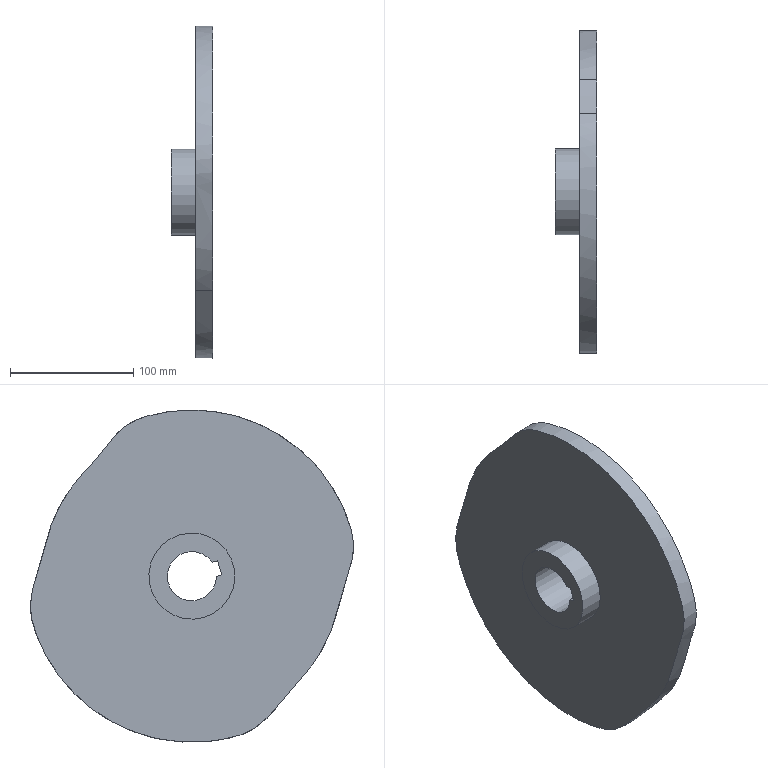Part | NX | features 146X000 2 | 1 solid | 11 faces | box 34 x 262.59 x 269.999 mm | volume 781015 mm3 | plane 6 | spline 3 | cylinder 2 | commonest cylinder face diameters 40 x1 70 x1
STEP:
#1=CARTESIAN_POINT('',(-21.5,-143.231,-819.079));
#2=VERTEX_POINT('',#1);
#3=CARTESIAN_POINT('',(-21.5,-138.999,-820.357));
#4=VERTEX_POINT('',#3);
#5=CARTESIAN_POINT('',(-21.5,-143.231,-819.079));
#6=DIRECTION('',(0.,0.9573,-0.2891));
#7=VECTOR('',#6,1000.);
#8=LINE('',#5,#7);
#9=EDGE_CURVE('',#2,#4,#8,.T.);
#10=ORIENTED_EDGE('',*,*,#9,.F.);
#11=CARTESIAN_POINT('',(12.5,-143.231,-819.079));
#12=VERTEX_POINT('',#11);
#13=CARTESIAN_POINT('',(-21.5,-143.231,-819.079));
#14=DIRECTION('',(1.,0.,0.));
#15=VECTOR('',#14,1000.);
#16=LINE('',#13,#15);
#17=EDGE_CURVE('',#2,#12,#16,.T.);
#18=ORIENTED_EDGE('',*,*,#17,.T.);
#19=CARTESIAN_POINT('',(12.5,-138.999,-820.357));
#20=VERTEX_POINT('',#19);
#21=CARTESIAN_POINT('',(12.5,-143.231,-819.079));
#22=DIRECTION('',(0.,0.9573,-0.2891));
#23=VECTOR('',#22,1000.);
#24=LINE('',#21,#23);
#25=EDGE_CURVE('',#12,#20,#24,.T.);
#26=ORIENTED_EDGE('',*,*,#25,.T.);
#27=CARTESIAN_POINT('',(-21.5,-138.999,-820.357));
#28=DIRECTION('',(1.,0.,0.));
#29=VECTOR('',#28,1000.);
#30=LINE('',#27,#29);
#31=EDGE_CURVE('',#4,#20,#30,.T.);
#32=ORIENTED_EDGE('',*,*,#31,.F.);
#33=EDGE_LOOP('',(#10,#18,#26,#32));
#34=FACE_BOUND('',#33,.T.);
#35=CARTESIAN_POINT('',(12.5,-143.231,-819.079));
#36=DIRECTION('',(0.,-0.2891,-0.9573));
#37=DIRECTION('',(0.,-0.9573,0.2891));
#38=AXIS2_PLACEMENT_3D('',#35,#36,#37);
#39=PLANE('',#38);
#40=ADVANCED_FACE('',(#34),#39,.F.);
#41=CARTESIAN_POINT('',(-21.5,-139.762,-807.591));
#42=VERTEX_POINT('',#41);
#43=CARTESIAN_POINT('',(-21.5,-139.762,-807.591));
#44=DIRECTION('',(0.,-0.2891,-0.9573));
#45=VECTOR('',#44,1000.);
#46=LINE('',#43,#45);
#47=EDGE_CURVE('',#42,#2,#46,.T.);
#48=ORIENTED_EDGE('',*,*,#47,.F.);
#49=CARTESIAN_POINT('',(12.5,-139.762,-807.591));
#50=VERTEX_POINT('',#49);
#51=CARTESIAN_POINT('',(-21.5,-139.762,-807.591));
#52=DIRECTION('',(1.,0.,0.));
#53=VECTOR('',#52,1000.);
#54=LINE('',#51,#53);
#55=EDGE_CURVE('',#42,#50,#54,.T.);
#56=ORIENTED_EDGE('',*,*,#55,.T.);
#57=CARTESIAN_POINT('',(12.5,-139.762,-807.591));
#58=DIRECTION('',(0.,-0.2891,-0.9573));
#59=VECTOR('',#58,1000.);
#60=LINE('',#57,#59);
#61=EDGE_CURVE('',#50,#12,#60,.T.);
#62=ORIENTED_EDGE('',*,*,#61,.T.);
#63=ORIENTED_EDGE('',*,*,#17,.F.);
#64=EDGE_LOOP('',(#48,#56,#62,#63));
#65=FACE_BOUND('',#64,.T.);
#66=CARTESIAN_POINT('',(12.5,-139.762,-807.591));
#67=DIRECTION('',(0.,-0.9573,0.2891));
#68=DIRECTION('',(-1.,0.,0.));
#69=AXIS2_PLACEMENT_3D('',#66,#67,#68);
#70=PLANE('',#69);
#71=ADVANCED_FACE('',(#65),#70,.F.);
#72=CARTESIAN_POINT('',(12.5,-135.529,-808.87));
#73=VERTEX_POINT('',#72);
#74=CARTESIAN_POINT('',(12.5,-135.529,-808.87));
#75=DIRECTION('',(0.,-0.9573,0.2891));
#76=VECTOR('',#75,1000.);
#77=LINE('',#74,#76);
#78=EDGE_CURVE('',#73,#50,#77,.T.);
#79=ORIENTED_EDGE('',*,*,#78,.T.);
#80=ORIENTED_EDGE('',*,*,#55,.F.);
#81=CARTESIAN_POINT('',(-21.5,-135.529,-808.87));
#82=VERTEX_POINT('',#81);
#83=CARTESIAN_POINT('',(-21.5,-135.529,-808.87));
#84=DIRECTION('',(0.,-0.9573,0.2891));
#85=VECTOR('',#84,1000.);
#86=LINE('',#83,#85);
#87=EDGE_CURVE('',#82,#42,#86,.T.);
#88=ORIENTED_EDGE('',*,*,#87,.F.);
#89=CARTESIAN_POINT('',(12.5,-135.529,-808.87));
#90=DIRECTION('',(-1.,0.,0.));
#91=VECTOR('',#90,1000.);
#92=LINE('',#89,#91);
#93=EDGE_CURVE('',#73,#82,#92,.T.);
#94=ORIENTED_EDGE('',*,*,#93,.F.);
#95=EDGE_LOOP('',(#79,#80,#88,#94));
#96=FACE_BOUND('',#95,.T.);
#97=CARTESIAN_POINT('',(12.5,-139.762,-807.591));
#98=DIRECTION('',(0.,0.2891,0.9573));
#99=DIRECTION('',(0.,0.9573,-0.2891));
#100=AXIS2_PLACEMENT_3D('',#97,#98,#99);
#101=PLANE('',#100);
#102=ADVANCED_FACE('',(#96),#101,.F.);
#103=CARTESIAN_POINT('',(-1.5,-129.119,-853.635));
#104=VERTEX_POINT('',#103);
#105=CARTESIAN_POINT('',(-1.5,-119.,-820.129));
#106=DIRECTION('',(1.,0.,0.));
#107=DIRECTION('',(0.,-0.2891,-0.9573));
#108=AXIS2_PLACEMENT_3D('',#105,#106,#107);
#109=CIRCLE('',#108,35.);
#110=EDGE_CURVE('',#104,#104,#109,.T.);
#111=ORIENTED_EDGE('',*,*,#110,.F.);
#112=EDGE_LOOP('',(#111));
#113=FACE_BOUND('',#112,.T.);
#114=CARTESIAN_POINT('',(-21.5,-108.881,-786.624));
#115=VERTEX_POINT('',#114);
#116=CARTESIAN_POINT('',(-21.5,-119.,-820.129));
#117=DIRECTION('',(-1.,0.,0.));
#118=DIRECTION('',(0.,0.2891,0.9573));
#119=AXIS2_PLACEMENT_3D('',#116,#117,#118);
#120=CIRCLE('',#119,35.);
#121=EDGE_CURVE('',#115,#115,#120,.T.);
#122=ORIENTED_EDGE('',*,*,#121,.F.);
#123=EDGE_LOOP('',(#122));
#124=FACE_BOUND('',#123,.T.);
#125=CARTESIAN_POINT('',(-21.5,-119.,-820.129));
#126=DIRECTION('',(1.,0.,0.));
#127=DIRECTION('',(0.,0.2891,0.9573));
#128=AXIS2_PLACEMENT_3D('',#125,#126,#127);
#129=CYLINDRICAL_SURFACE('',#128,35.);
#130=ADVANCED_FACE('',(#113,#124),#129,.T.);
#131=ORIENTED_EDGE('',*,*,#47,.T.);
#132=ORIENTED_EDGE('',*,*,#9,.T.);
#133=CARTESIAN_POINT('',(-21.5,-119.,-820.129));
#134=DIRECTION('',(1.,0.,0.));
#135=DIRECTION('',(0.,-0.9999,-0.01138));
#136=AXIS2_PLACEMENT_3D('',#133,#134,#135);
#137=CIRCLE('',#136,20.);
#138=EDGE_CURVE('',#4,#82,#137,.T.);
#139=ORIENTED_EDGE('',*,*,#138,.T.);
#140=ORIENTED_EDGE('',*,*,#87,.T.);
#141=EDGE_LOOP('',(#131,#132,#139,#140));
#142=FACE_BOUND('',#141,.T.);
#143=ORIENTED_EDGE('',*,*,#121,.T.);
#144=EDGE_LOOP('',(#143));
#145=FACE_BOUND('',#144,.T.);
#146=CARTESIAN_POINT('',(-21.5,-119.,-820.129));
#147=DIRECTION('',(-1.,0.,0.));
#148=DIRECTION('',(0.,-0.2891,-0.9573));
#149=AXIS2_PLACEMENT_3D('',#146,#147,#148);
#150=PLANE('',#149);
#151=ADVANCED_FACE('',(#142,#145),#150,.T.);
#152=ORIENTED_EDGE('',*,*,#138,.F.);
#153=ORIENTED_EDGE('',*,*,#31,.T.);
#154=CARTESIAN_POINT('',(12.5,-119.,-820.129));
#155=DIRECTION('',(-1.,0.,0.));
#156=DIRECTION('',(0.,-0.2891,-0.9573));
#157=AXIS2_PLACEMENT_3D('',#154,#155,#156);
#158=CIRCLE('',#157,20.);
#159=EDGE_CURVE('',#73,#20,#158,.T.);
#160=ORIENTED_EDGE('',*,*,#159,.F.);
#161=ORIENTED_EDGE('',*,*,#93,.T.);
#162=EDGE_LOOP('',(#152,#153,#160,#161));
#163=FACE_BOUND('',#162,.T.);
#164=CARTESIAN_POINT('',(-1.5,-119.,-820.129));
#165=DIRECTION('',(1.,0.,0.));
#166=DIRECTION('',(0.,0.2891,0.9573));
#167=AXIS2_PLACEMENT_3D('',#164,#165,#166);
#168=CYLINDRICAL_SURFACE('',#167,20.);
#169=ADVANCED_FACE('',(#163),#168,.F.);
#170=ORIENTED_EDGE('',*,*,#25,.F.);
#171=ORIENTED_EDGE('',*,*,#61,.F.);
#172=ORIENTED_EDGE('',*,*,#78,.F.);
#173=ORIENTED_EDGE('',*,*,#159,.T.);
#174=EDGE_LOOP('',(#170,#171,#172,#173));
#175=FACE_BOUND('',#174,.T.);
#176=CARTESIAN_POINT('',(12.5,-55.289,-707.283));
#177=VERTEX_POINT('',#176);
#178=CARTESIAN_POINT('',(12.5,-210.557,-900.047));
#179=VERTEX_POINT('',#178);
#180=CARTESIAN_POINT('',(12.5,-210.557,-900.047));
#181=CARTESIAN_POINT('',(12.5,-215.628,-894.239));
#182=CARTESIAN_POINT('',(12.5,-222.402,-884.799));
#183=CARTESIAN_POINT('',(12.5,-229.525,-871.101));
#184=CARTESIAN_POINT('',(12.5,-233.877,-860.369));
#185=CARTESIAN_POINT('',(12.5,-236.603,-851.114));
#186=CARTESIAN_POINT('',(12.5,-238.326,-843.598));
#187=CARTESIAN_POINT('',(12.5,-240.291,-836.142));
#188=CARTESIAN_POINT('',(12.5,-242.992,-826.89));
#189=CARTESIAN_POINT('',(12.5,-245.919,-817.711));
#190=CARTESIAN_POINT('',(12.5,-248.427,-810.413));
#191=CARTESIAN_POINT('',(12.5,-249.773,-804.781));
#192=CARTESIAN_POINT('',(12.5,-250.436,-799.023));
#193=CARTESIAN_POINT('',(12.5,-250.459,-793.232));
#194=CARTESIAN_POINT('',(12.5,-249.844,-787.468));
#195=CARTESIAN_POINT('',(12.5,-248.527,-781.829));
#196=CARTESIAN_POINT('',(12.5,-246.734,-776.328));
#197=CARTESIAN_POINT('',(12.5,-244.086,-769.086));
#198=CARTESIAN_POINT('',(12.5,-240.183,-760.263));
#199=CARTESIAN_POINT('',(12.5,-232.763,-746.73));
#200=CARTESIAN_POINT('',(12.5,-221.361,-731.099));
#201=CARTESIAN_POINT('',(12.5,-204.681,-714.949));
#202=CARTESIAN_POINT('',(12.5,-185.491,-701.879));
#203=CARTESIAN_POINT('',(12.5,-164.354,-692.273));
#204=CARTESIAN_POINT('',(12.5,-141.888,-686.412));
#205=CARTESIAN_POINT('',(12.5,-122.608,-684.792));
#206=CARTESIAN_POINT('',(12.5,-107.189,-685.481));
#207=CARTESIAN_POINT('',(12.5,-95.708,-686.986));
#208=CARTESIAN_POINT('',(12.5,-84.41,-689.462));
#209=CARTESIAN_POINT('',(12.5,-73.316,-692.896));
#210=CARTESIAN_POINT('',(12.5,-63.345,-698.946));
#211=CARTESIAN_POINT('',(12.5,-57.75,-704.315));
#212=CARTESIAN_POINT('',(12.5,-55.289,-707.283));
#213=B_SPLINE_CURVE_WITH_KNOTS('',3,(#180,#181,#182,#183,#184,#185,#186,#187,#188,#189,#190,#191,#192,#193,#194,#195,#196,#197,#198,#199,#200,#201,#202,#203,#204,#205,#206,#207,#208,#209,#210,#211,#212),.UNSPECIFIED.,.F.,.F.,(4,1,1,1,1,1,1,1,1,1,1,1,1,1,1,1,1,1,1,1,1,1,1,1,1,1,1,1,1,1,4),(0.,0.0625,0.09375,0.125,0.1562,0.1719,0.1875,0.2188,0.25,0.2656,0.2812,0.2969,0.3125,0.3281,0.3438,0.3594,0.375,0.4062,0.4375,0.5,0.5625,0.625,0.6875,0.75,0.8125,0.8438,0.875,0.9062,0.9375,0.9688,1.),.UNSPECIFIED.);
#214=EDGE_CURVE('',#177,#179,#213,.F.);
#215=ORIENTED_EDGE('',*,*,#214,.T.);
#216=CARTESIAN_POINT('',(12.5,-28.192,-739.361));
#217=VERTEX_POINT('',#216);
#218=CARTESIAN_POINT('',(12.5,-28.192,-739.361));
#219=CARTESIAN_POINT('',(12.5,-22.457,-745.808));
#220=CARTESIAN_POINT('',(12.5,-14.889,-756.399));
#221=CARTESIAN_POINT('',(12.5,-7.211,-771.882));
#222=CARTESIAN_POINT('',(12.5,-3.46,-782.011));
#223=CARTESIAN_POINT('',(12.5,-1.129,-790.322));
#224=CARTESIAN_POINT('',(12.5,0.8153,-798.73));
#225=CARTESIAN_POINT('',(12.5,3.97,-809.049));
#226=CARTESIAN_POINT('',(12.5,8.02,-821.337));
#227=CARTESIAN_POINT('',(12.5,11.36,-833.86));
#228=CARTESIAN_POINT('',(12.5,12.469,-844.644));
#229=CARTESIAN_POINT('',(12.5,11.752,-853.272));
#230=CARTESIAN_POINT('',(12.5,10.214,-859.571));
#231=CARTESIAN_POINT('',(12.5,8.118,-865.696));
#232=CARTESIAN_POINT('',(12.5,5.031,-873.754));
#233=CARTESIAN_POINT('',(12.5,0.4236,-883.52));
#234=CARTESIAN_POINT('',(12.5,-6.192,-894.661));
#235=CARTESIAN_POINT('',(12.5,-16.394,-908.605));
#236=CARTESIAN_POINT('',(12.5,-31.568,-924.078));
#237=CARTESIAN_POINT('',(12.5,-52.981,-938.835));
#238=CARTESIAN_POINT('',(12.5,-76.814,-949.242));
#239=CARTESIAN_POINT('',(12.5,-97.963,-953.968));
#240=CARTESIAN_POINT('',(12.5,-115.19,-955.283));
#241=CARTESIAN_POINT('',(12.5,-128.143,-955.022));
#242=CARTESIAN_POINT('',(12.5,-141.019,-953.545));
#243=CARTESIAN_POINT('',(12.5,-151.558,-951.228));
#244=CARTESIAN_POINT('',(12.5,-159.879,-948.915));
#245=CARTESIAN_POINT('',(12.5,-167.825,-945.483));
#246=CARTESIAN_POINT('',(12.5,-176.675,-939.179));
#247=CARTESIAN_POINT('',(12.5,-185.649,-929.812));
#248=CARTESIAN_POINT('',(12.5,-193.715,-919.69));
#249=CARTESIAN_POINT('',(12.5,-201.826,-909.605));
#250=CARTESIAN_POINT('',(12.5,-207.604,-903.192));
#251=CARTESIAN_POINT('',(12.5,-210.557,-900.047));
#252=B_SPLINE_CURVE_WITH_KNOTS('',3,(#218,#219,#220,#221,#222,#223,#224,#225,#226,#227,#228,#229,#230,#231,#232,#233,#234,#235,#236,#237,#238,#239,#240,#241,#242,#243,#244,#245,#246,#247,#248,#249,#250,#251),.UNSPECIFIED.,.F.,.F.,(4,1,1,1,1,1,1,1,1,1,1,1,1,1,1,1,1,1,1,1,1,1,1,1,1,1,1,1,1,1,1,4),(0.,0.0625,0.09375,0.125,0.1406,0.1562,0.1875,0.2188,0.25,0.2812,0.2969,0.3125,0.3281,0.3438,0.375,0.4062,0.4375,0.5,0.5625,0.625,0.6875,0.7188,0.75,0.7812,0.8125,0.8281,0.8438,0.875,0.9062,0.9375,0.9688,1.),.UNSPECIFIED.);
#253=EDGE_CURVE('',#179,#217,#252,.F.);
#254=ORIENTED_EDGE('',*,*,#253,.T.);
#255=CARTESIAN_POINT('',(12.5,-55.289,-707.283));
#256=CARTESIAN_POINT('',(12.5,-46.692,-718.331));
#257=CARTESIAN_POINT('',(12.5,-37.848,-729.212));
#258=CARTESIAN_POINT('',(12.5,-28.192,-739.361));
#259=B_SPLINE_CURVE_WITH_KNOTS('',3,(#255,#256,#257,#258),.UNSPECIFIED.,.F.,.F.,(4,4),(0.,1.),.UNSPECIFIED.);
#260=EDGE_CURVE('',#217,#177,#259,.F.);
#261=ORIENTED_EDGE('',*,*,#260,.T.);
#262=EDGE_LOOP('',(#215,#254,#261));
#263=FACE_BOUND('',#262,.T.);
#264=CARTESIAN_POINT('',(12.5,-258.55,-814.638));
#265=DIRECTION('',(-1.,0.,0.));
#266=DIRECTION('',(0.,-0.2891,-0.9573));
#267=AXIS2_PLACEMENT_3D('',#264,#265,#266);
#268=PLANE('',#267);
#269=ADVANCED_FACE('',(#175,#263),#268,.F.);
#270=ORIENTED_EDGE('',*,*,#253,.F.);
#271=CARTESIAN_POINT('',(-1.5,-210.557,-900.047));
#272=VERTEX_POINT('',#271);
#273=CARTESIAN_POINT('',(12.96,-210.557,-900.047));
#274=DIRECTION('',(-1.,0.,0.));
#275=VECTOR('',#274,1000.);
#276=LINE('',#273,#275);
#277=EDGE_CURVE('',#272,#179,#276,.F.);
#278=ORIENTED_EDGE('',*,*,#277,.F.);
#279=CARTESIAN_POINT('',(-1.5,-28.192,-739.361));
#280=VERTEX_POINT('',#279);
#281=CARTESIAN_POINT('',(-1.5,-210.557,-900.047));
#282=CARTESIAN_POINT('',(-1.5,-207.605,-903.192));
#283=CARTESIAN_POINT('',(-1.5,-201.825,-909.604));
#284=CARTESIAN_POINT('',(-1.5,-193.716,-919.69));
#285=CARTESIAN_POINT('',(-1.5,-185.649,-929.812));
#286=CARTESIAN_POINT('',(-1.5,-176.676,-939.179));
#287=CARTESIAN_POINT('',(-1.5,-167.825,-945.482));
#288=CARTESIAN_POINT('',(-1.5,-159.88,-948.917));
#289=CARTESIAN_POINT('',(-1.5,-151.557,-951.228));
#290=CARTESIAN_POINT('',(-1.5,-141.019,-953.545));
#291=CARTESIAN_POINT('',(-1.5,-128.143,-955.022));
#292=CARTESIAN_POINT('',(-1.5,-115.189,-955.283));
#293=CARTESIAN_POINT('',(-1.5,-97.961,-953.968));
#294=CARTESIAN_POINT('',(-1.5,-76.812,-949.241));
#295=CARTESIAN_POINT('',(-1.5,-52.98,-938.835));
#296=CARTESIAN_POINT('',(-1.5,-31.567,-924.077));
#297=CARTESIAN_POINT('',(-1.5,-16.394,-908.604));
#298=CARTESIAN_POINT('',(-1.5,-6.192,-894.66));
#299=CARTESIAN_POINT('',(-1.5,0.4238,-883.52));
#300=CARTESIAN_POINT('',(-1.5,5.032,-873.754));
#301=CARTESIAN_POINT('',(-1.5,8.118,-865.696));
#302=CARTESIAN_POINT('',(-1.5,10.217,-859.571));
#303=CARTESIAN_POINT('',(-1.5,11.752,-853.272));
#304=CARTESIAN_POINT('',(-1.5,12.469,-844.644));
#305=CARTESIAN_POINT('',(-1.5,11.36,-833.859));
#306=CARTESIAN_POINT('',(-1.5,8.02,-821.336));
#307=CARTESIAN_POINT('',(-1.5,3.97,-809.049));
#308=CARTESIAN_POINT('',(-1.5,0.8134,-798.73));
#309=CARTESIAN_POINT('',(-1.5,-1.13,-790.322));
#310=CARTESIAN_POINT('',(-1.5,-3.46,-782.011));
#311=CARTESIAN_POINT('',(-1.5,-7.211,-771.882));
#312=CARTESIAN_POINT('',(-1.5,-14.889,-756.399));
#313=CARTESIAN_POINT('',(-1.5,-22.457,-745.808));
#314=CARTESIAN_POINT('',(-1.5,-28.192,-739.361));
#315=B_SPLINE_CURVE_WITH_KNOTS('',3,(#281,#282,#283,#284,#285,#286,#287,#288,#289,#290,#291,#292,#293,#294,#295,#296,#297,#298,#299,#300,#301,#302,#303,#304,#305,#306,#307,#308,#309,#310,#311,#312,#313,#314),.UNSPECIFIED.,.F.,.F.,(4,1,1,1,1,1,1,1,1,1,1,1,1,1,1,1,1,1,1,1,1,1,1,1,1,1,1,1,1,1,1,4),(0.,0.03125,0.0625,0.09375,0.125,0.1562,0.1719,0.1875,0.2188,0.25,0.2812,0.3125,0.375,0.4375,0.5,0.5625,0.5938,0.625,0.6562,0.6719,0.6875,0.7031,0.7188,0.75,0.7812,0.8125,0.8438,0.8594,0.875,0.9062,0.9375,1.),.UNSPECIFIED.);
#316=EDGE_CURVE('',#280,#272,#315,.F.);
#317=ORIENTED_EDGE('',*,*,#316,.F.);
#318=CARTESIAN_POINT('',(12.96,-28.192,-739.361));
#319=DIRECTION('',(-1.,0.,0.));
#320=VECTOR('',#319,1000.);
#321=LINE('',#318,#320);
#322=EDGE_CURVE('',#280,#217,#321,.F.);
#323=ORIENTED_EDGE('',*,*,#322,.T.);
#324=EDGE_LOOP('',(#270,#278,#317,#323));
#325=FACE_BOUND('',#324,.T.);
#326=CARTESIAN_POINT('',(12.5,-28.192,-739.361));
#327=CARTESIAN_POINT('',(-1.5,-28.192,-739.361));
#328=CARTESIAN_POINT('',(12.5,-22.772,-745.455));
#329=CARTESIAN_POINT('',(-1.5,-22.772,-745.455));
#330=CARTESIAN_POINT('',(12.5,-15.496,-755.509));
#331=CARTESIAN_POINT('',(-1.5,-15.496,-755.509));
#332=CARTESIAN_POINT('',(12.5,-7.956,-770.227));
#333=CARTESIAN_POINT('',(-1.5,-7.956,-770.227));
#334=CARTESIAN_POINT('',(12.5,-4.229,-779.831));
#335=CARTESIAN_POINT('',(-1.5,-4.229,-779.831));
#336=CARTESIAN_POINT('',(12.5,-1.82,-787.656));
#337=CARTESIAN_POINT('',(-1.5,-1.82,-787.656));
#338=CARTESIAN_POINT('',(12.5,-0.405,-793.602));
#339=CARTESIAN_POINT('',(-1.5,-0.405,-793.602));
#340=CARTESIAN_POINT('',(12.5,1.116,-799.529));
#341=CARTESIAN_POINT('',(-1.5,1.116,-799.529));
#342=CARTESIAN_POINT('',(12.5,3.433,-807.345));
#343=CARTESIAN_POINT('',(-1.5,3.433,-807.345));
#344=CARTESIAN_POINT('',(12.5,6.621,-817.038));
#345=CARTESIAN_POINT('',(-1.5,6.621,-817.038));
#346=CARTESIAN_POINT('',(12.5,10.143,-828.727));
#347=CARTESIAN_POINT('',(-1.5,10.143,-828.727));
#348=CARTESIAN_POINT('',(12.5,11.998,-838.828));
#349=CARTESIAN_POINT('',(-1.5,11.998,-838.828));
#350=CARTESIAN_POINT('',(12.5,12.271,-846.909));
#351=CARTESIAN_POINT('',(-1.5,12.271,-846.909));
#352=CARTESIAN_POINT('',(12.5,11.771,-853.026));
#353=CARTESIAN_POINT('',(-1.5,11.771,-853.026));
#354=CARTESIAN_POINT('',(12.5,10.378,-859.029));
#355=CARTESIAN_POINT('',(-1.5,10.378,-859.029));
#356=CARTESIAN_POINT('',(12.5,7.74,-866.863));
#357=CARTESIAN_POINT('',(-1.5,7.74,-866.863));
#358=CARTESIAN_POINT('',(12.5,3.793,-876.75));
#359=CARTESIAN_POINT('',(-1.5,3.793,-876.75));
#360=CARTESIAN_POINT('',(12.5,-2.309,-888.442));
#361=CARTESIAN_POINT('',(-1.5,-2.309,-888.442));
#362=CARTESIAN_POINT('',(12.5,-12.196,-903.583));
#363=CARTESIAN_POINT('',(-1.5,-12.196,-903.583));
#364=CARTESIAN_POINT('',(12.5,-27.872,-921.093));
#365=CARTESIAN_POINT('',(-1.5,-27.872,-921.093));
#366=CARTESIAN_POINT('',(12.5,-51.286,-938.117));
#367=CARTESIAN_POINT('',(-1.5,-51.286,-938.117));
#368=CARTESIAN_POINT('',(12.5,-77.88,-949.785));
#369=CARTESIAN_POINT('',(-1.5,-77.88,-949.785));
#370=CARTESIAN_POINT('',(12.5,-101.127,-954.5));
#371=CARTESIAN_POINT('',(-1.5,-101.127,-954.5));
#372=CARTESIAN_POINT('',(12.5,-119.427,-955.354));
#373=CARTESIAN_POINT('',(-1.5,-119.427,-955.354));
#374=CARTESIAN_POINT('',(12.5,-132.808,-954.636));
#375=CARTESIAN_POINT('',(-1.5,-132.808,-954.636));
#376=CARTESIAN_POINT('',(12.5,-143.516,-953.009));
#377=CARTESIAN_POINT('',(-1.5,-143.516,-953.009));
#378=CARTESIAN_POINT('',(12.5,-151.748,-951.136));
#379=CARTESIAN_POINT('',(-1.5,-151.748,-951.136));
#380=CARTESIAN_POINT('',(12.5,-157.76,-949.537));
#381=CARTESIAN_POINT('',(-1.5,-157.76,-949.537));
#382=CARTESIAN_POINT('',(12.5,-163.513,-947.468));
#383=CARTESIAN_POINT('',(-1.5,-163.513,-947.468));
#384=CARTESIAN_POINT('',(12.5,-170.642,-943.635));
#385=CARTESIAN_POINT('',(-1.5,-170.642,-943.635));
#386=CARTESIAN_POINT('',(12.5,-178.706,-937.247));
#387=CARTESIAN_POINT('',(-1.5,-178.706,-937.247));
#388=CARTESIAN_POINT('',(12.5,-186.94,-928.233));
#389=CARTESIAN_POINT('',(-1.5,-186.94,-928.233));
#390=CARTESIAN_POINT('',(12.5,-194.567,-918.616));
#391=CARTESIAN_POINT('',(-1.5,-194.567,-918.616));
#392=CARTESIAN_POINT('',(12.5,-200.969,-910.663));
#393=CARTESIAN_POINT('',(-1.5,-200.969,-910.663));
#394=CARTESIAN_POINT('',(12.5,-206.404,-904.557));
#395=CARTESIAN_POINT('',(-1.5,-206.404,-904.557));
#396=CARTESIAN_POINT('',(12.5,-209.213,-901.587));
#397=CARTESIAN_POINT('',(-1.5,-209.213,-901.587));
#398=CARTESIAN_POINT('',(12.5,-210.557,-900.047));
#399=CARTESIAN_POINT('',(-1.5,-210.557,-900.047));
#400=B_SPLINE_SURFACE_WITH_KNOTS('',3,1,((#326,#327),(#328,#329),(#330,#331),(#332,#333),(#334,#335),(#336,#337),(#338,#339),(#340,#341),(#342,#343),(#344,#345),(#346,#347),(#348,#349),(#350,#351),(#352,#353),(#354,#355),(#356,#357),(#358,#359),(#360,#361),(#362,#363),(#364,#365),(#366,#367),(#368,#369),(#370,#371),(#372,#373),(#374,#375),(#376,#377),(#378,#379),(#380,#381),(#382,#383),(#384,#385),(#386,#387),(#388,#389),(#390,#391),(#392,#393),(#394,#395),(#396,#397),(#398,#399)),.SURF_OF_LINEAR_EXTRUSION.,.F.,.F.,.F.,(4,1,1,1,1,1,1,1,1,1,1,1,1,1,1,1,1,1,1,1,1,1,1,1,1,1,1,1,1,1,1,1,1,1,4),(2,2),(0.01026,0.0709,0.1012,0.1315,0.1467,0.1619,0.177,0.1922,0.2225,0.2528,0.2832,0.2983,0.3135,0.3286,0.3438,0.3741,0.4045,0.4348,0.4954,0.5561,0.6167,0.6774,0.7077,0.738,0.7683,0.7835,0.7987,0.8138,0.829,0.8593,0.8896,0.9199,0.9503,0.9654,0.9806),(0.,1.),.UNSPECIFIED.);
#401=ADVANCED_FACE('',(#325),#400,.T.);
#402=ORIENTED_EDGE('',*,*,#260,.F.);
#403=ORIENTED_EDGE('',*,*,#322,.F.);
#404=CARTESIAN_POINT('',(-1.5,-55.289,-707.283));
#405=VERTEX_POINT('',#404);
#406=CARTESIAN_POINT('',(-1.5,-28.192,-739.361));
#407=CARTESIAN_POINT('',(-1.5,-37.848,-729.212));
#408=CARTESIAN_POINT('',(-1.5,-46.692,-718.331));
#409=CARTESIAN_POINT('',(-1.5,-55.289,-707.283));
#410=B_SPLINE_CURVE_WITH_KNOTS('',3,(#406,#407,#408,#409),.UNSPECIFIED.,.F.,.F.,(4,4),(0.,1.),.UNSPECIFIED.);
#411=EDGE_CURVE('',#405,#280,#410,.F.);
#412=ORIENTED_EDGE('',*,*,#411,.F.);
#413=CARTESIAN_POINT('',(12.96,-55.289,-707.283));
#414=DIRECTION('',(-1.,0.,0.));
#415=VECTOR('',#414,1000.);
#416=LINE('',#413,#415);
#417=EDGE_CURVE('',#177,#405,#416,.T.);
#418=ORIENTED_EDGE('',*,*,#417,.F.);
#419=EDGE_LOOP('',(#402,#403,#412,#418));
#420=FACE_BOUND('',#419,.T.);
#421=CARTESIAN_POINT('',(12.5,-55.289,-707.283));
#422=CARTESIAN_POINT('',(-1.5,-55.289,-707.283));
#423=CARTESIAN_POINT('',(12.5,-54.177,-708.63));
#424=CARTESIAN_POINT('',(-1.5,-54.177,-708.63));
#425=CARTESIAN_POINT('',(12.5,-52.051,-711.419));
#426=CARTESIAN_POINT('',(-1.5,-52.051,-711.419));
#427=CARTESIAN_POINT('',(12.5,-47.694,-716.899));
#428=CARTESIAN_POINT('',(-1.5,-47.694,-716.899));
#429=CARTESIAN_POINT('',(12.5,-42.178,-723.693));
#430=CARTESIAN_POINT('',(-1.5,-42.178,-723.693));
#431=CARTESIAN_POINT('',(12.5,-35.355,-731.674));
#432=CARTESIAN_POINT('',(-1.5,-35.355,-731.674));
#433=CARTESIAN_POINT('',(12.5,-30.52,-736.745));
#434=CARTESIAN_POINT('',(-1.5,-30.52,-736.745));
#435=CARTESIAN_POINT('',(12.5,-28.192,-739.361));
#436=CARTESIAN_POINT('',(-1.5,-28.192,-739.361));
#437=B_SPLINE_SURFACE_WITH_KNOTS('',3,1,((#421,#422),(#423,#424),(#425,#426),(#427,#428),(#429,#430),(#431,#432),(#433,#434),(#435,#436)),.SURF_OF_LINEAR_EXTRUSION.,.F.,.F.,.F.,(4,1,1,1,1,4),(2,2),(0.009829,0.1324,0.2549,0.5,0.7451,0.9902),(0.,1.),.UNSPECIFIED.);
#438=ADVANCED_FACE('',(#420),#437,.T.);
#439=CARTESIAN_POINT('',(-1.5,-55.289,-707.283));
#440=CARTESIAN_POINT('',(-1.5,-57.75,-704.315));
#441=CARTESIAN_POINT('',(-1.5,-63.345,-698.947));
#442=CARTESIAN_POINT('',(-1.5,-73.314,-692.896));
#443=CARTESIAN_POINT('',(-1.5,-84.409,-689.474));
#444=CARTESIAN_POINT('',(-1.5,-95.704,-686.985));
#445=CARTESIAN_POINT('',(-1.5,-107.185,-685.482));
#446=CARTESIAN_POINT('',(-1.5,-122.604,-684.794));
#447=CARTESIAN_POINT('',(-1.5,-141.885,-686.413));
#448=CARTESIAN_POINT('',(-1.5,-164.351,-692.273));
#449=CARTESIAN_POINT('',(-1.5,-185.489,-701.878));
#450=CARTESIAN_POINT('',(-1.5,-204.68,-714.947));
#451=CARTESIAN_POINT('',(-1.5,-221.359,-731.098));
#452=CARTESIAN_POINT('',(-1.5,-232.762,-746.73));
#453=CARTESIAN_POINT('',(-1.5,-240.182,-760.264));
#454=CARTESIAN_POINT('',(-1.5,-244.093,-769.085));
#455=CARTESIAN_POINT('',(-1.5,-246.724,-776.332));
#456=CARTESIAN_POINT('',(-1.5,-248.544,-781.825));
#457=CARTESIAN_POINT('',(-1.5,-249.837,-787.471));
#458=CARTESIAN_POINT('',(-1.5,-250.461,-793.231));
#459=CARTESIAN_POINT('',(-1.5,-250.437,-799.023));
#460=CARTESIAN_POINT('',(-1.5,-249.771,-804.779));
#461=CARTESIAN_POINT('',(-1.5,-248.431,-810.415));
#462=CARTESIAN_POINT('',(-1.5,-245.915,-817.707));
#463=CARTESIAN_POINT('',(-1.5,-242.998,-826.89));
#464=CARTESIAN_POINT('',(-1.5,-240.278,-836.138));
#465=CARTESIAN_POINT('',(-1.5,-238.337,-843.6));
#466=CARTESIAN_POINT('',(-1.5,-236.602,-851.112));
#467=CARTESIAN_POINT('',(-1.5,-233.876,-860.368));
#468=CARTESIAN_POINT('',(-1.5,-229.523,-871.1));
#469=CARTESIAN_POINT('',(-1.5,-222.403,-884.798));
#470=CARTESIAN_POINT('',(-1.5,-215.627,-894.238));
#471=CARTESIAN_POINT('',(-1.5,-210.557,-900.047));
#472=B_SPLINE_CURVE_WITH_KNOTS('',3,(#439,#440,#441,#442,#443,#444,#445,#446,#447,#448,#449,#450,#451,#452,#453,#454,#455,#456,#457,#458,#459,#460,#461,#462,#463,#464,#465,#466,#467,#468,#469,#470,#471),.UNSPECIFIED.,.F.,.F.,(4,1,1,1,1,1,1,1,1,1,1,1,1,1,1,1,1,1,1,1,1,1,1,1,1,1,1,1,1,1,4),(0.,0.03125,0.0625,0.09375,0.125,0.1562,0.1875,0.25,0.3125,0.375,0.4375,0.5,0.5625,0.5938,0.625,0.6406,0.6562,0.6719,0.6875,0.7031,0.7188,0.7344,0.75,0.7812,0.8125,0.8281,0.8438,0.875,0.9062,0.9375,1.),.UNSPECIFIED.);
#473=EDGE_CURVE('',#272,#405,#472,.F.);
#474=ORIENTED_EDGE('',*,*,#473,.F.);
#475=ORIENTED_EDGE('',*,*,#277,.T.);
#476=ORIENTED_EDGE('',*,*,#214,.F.);
#477=ORIENTED_EDGE('',*,*,#417,.T.);
#478=EDGE_LOOP('',(#474,#475,#476,#477));
#479=FACE_BOUND('',#478,.T.);
#480=CARTESIAN_POINT('',(12.5,-210.557,-900.047));
#481=CARTESIAN_POINT('',(-1.5,-210.557,-900.047));
#482=CARTESIAN_POINT('',(12.5,-215.321,-894.59));
#483=CARTESIAN_POINT('',(-1.5,-215.321,-894.59));
#484=CARTESIAN_POINT('',(12.5,-221.801,-885.671));
#485=CARTESIAN_POINT('',(-1.5,-221.801,-885.671));
#486=CARTESIAN_POINT('',(12.5,-228.741,-872.73));
#487=CARTESIAN_POINT('',(-1.5,-228.741,-872.73));
#488=CARTESIAN_POINT('',(12.5,-233.034,-862.61));
#489=CARTESIAN_POINT('',(-1.5,-233.034,-862.61));
#490=CARTESIAN_POINT('',(12.5,-236.392,-852.218));
#491=CARTESIAN_POINT('',(-1.5,-236.392,-852.218));
#492=CARTESIAN_POINT('',(12.5,-238.76,-841.616));
#493=CARTESIAN_POINT('',(-1.5,-238.76,-841.616));
#494=CARTESIAN_POINT('',(12.5,-241.706,-831.154));
#495=CARTESIAN_POINT('',(-1.5,-241.706,-831.154));
#496=CARTESIAN_POINT('',(12.5,-244.402,-822.507));
#497=CARTESIAN_POINT('',(-1.5,-244.402,-822.507));
#498=CARTESIAN_POINT('',(12.5,-246.624,-815.606));
#499=CARTESIAN_POINT('',(-1.5,-246.624,-815.606));
#500=CARTESIAN_POINT('',(12.5,-248.418,-810.471));
#501=CARTESIAN_POINT('',(-1.5,-248.418,-810.471));
#502=CARTESIAN_POINT('',(12.5,-249.684,-805.172));
#503=CARTESIAN_POINT('',(-1.5,-249.684,-805.172));
#504=CARTESIAN_POINT('',(12.5,-250.607,-797.926));
#505=CARTESIAN_POINT('',(-1.5,-250.607,-797.926));
#506=CARTESIAN_POINT('',(12.5,-250.386,-790.744));
#507=CARTESIAN_POINT('',(-1.5,-250.386,-790.744));
#508=CARTESIAN_POINT('',(12.5,-249.013,-783.545));
#509=CARTESIAN_POINT('',(-1.5,-249.013,-783.545));
#510=CARTESIAN_POINT('',(12.5,-246.861,-776.585));
#511=CARTESIAN_POINT('',(-1.5,-246.861,-776.585));
#512=CARTESIAN_POINT('',(12.5,-243.634,-767.827));
#513=CARTESIAN_POINT('',(-1.5,-243.634,-767.827));
#514=CARTESIAN_POINT('',(12.5,-237.091,-753.914));
#515=CARTESIAN_POINT('',(-1.5,-237.091,-753.914));
#516=CARTESIAN_POINT('',(12.5,-226.305,-736.989));
#517=CARTESIAN_POINT('',(-1.5,-226.305,-736.989));
#518=CARTESIAN_POINT('',(12.5,-209.243,-718.663));
#519=CARTESIAN_POINT('',(-1.5,-209.243,-718.663));
#520=CARTESIAN_POINT('',(12.5,-188.607,-703.512));
#521=CARTESIAN_POINT('',(-1.5,-188.607,-703.512));
#522=CARTESIAN_POINT('',(12.5,-165.378,-692.491));
#523=CARTESIAN_POINT('',(-1.5,-165.378,-692.491));
#524=CARTESIAN_POINT('',(12.5,-140.834,-686.128));
#525=CARTESIAN_POINT('',(-1.5,-140.834,-686.128));
#526=CARTESIAN_POINT('',(12.5,-120.403,-684.728));
#527=CARTESIAN_POINT('',(-1.5,-120.403,-684.728));
#528=CARTESIAN_POINT('',(12.5,-104.66,-685.724));
#529=CARTESIAN_POINT('',(-1.5,-104.66,-685.724));
#530=CARTESIAN_POINT('',(12.5,-93.274,-687.439));
#531=CARTESIAN_POINT('',(-1.5,-93.274,-687.439));
#532=CARTESIAN_POINT('',(12.5,-84.226,-689.605));
#533=CARTESIAN_POINT('',(-1.5,-84.226,-689.605));
#534=CARTESIAN_POINT('',(12.5,-77.232,-691.697));
#535=CARTESIAN_POINT('',(-1.5,-77.232,-691.697));
#536=CARTESIAN_POINT('',(12.5,-70.573,-694.536));
#537=CARTESIAN_POINT('',(-1.5,-70.573,-694.536));
#538=CARTESIAN_POINT('',(12.5,-62.816,-699.409));
#539=CARTESIAN_POINT('',(-1.5,-62.816,-699.409));
#540=CARTESIAN_POINT('',(12.5,-57.601,-704.483));
#541=CARTESIAN_POINT('',(-1.5,-57.601,-704.483));
#542=CARTESIAN_POINT('',(12.5,-55.289,-707.283));
#543=CARTESIAN_POINT('',(-1.5,-55.289,-707.283));
#544=B_SPLINE_SURFACE_WITH_KNOTS('',3,1,((#480,#481),(#482,#483),(#484,#485),(#486,#487),(#488,#489),(#490,#491),(#492,#493),(#494,#495),(#496,#497),(#498,#499),(#500,#501),(#502,#503),(#504,#505),(#506,#507),(#508,#509),(#510,#511),(#512,#513),(#514,#515),(#516,#517),(#518,#519),(#520,#521),(#522,#523),(#524,#525),(#526,#527),(#528,#529),(#530,#531),(#532,#533),(#534,#535),(#536,#537),(#538,#539),(#540,#541),(#542,#543)),.SURF_OF_LINEAR_EXTRUSION.,.F.,.F.,.F.,(4,1,1,1,1,1,1,1,1,1,1,1,1,1,1,1,1,1,1,1,1,1,1,1,1,1,1,1,1,4),(2,2),(0.01044,0.07164,0.1022,0.1328,0.1634,0.194,0.2246,0.2552,0.2705,0.2858,0.3011,0.3164,0.347,0.3623,0.3776,0.4082,0.4388,0.5,0.5612,0.6224,0.6836,0.7448,0.806,0.8366,0.8672,0.8978,0.9131,0.9284,0.959,0.9896),(0.,1.),.UNSPECIFIED.);
#545=ADVANCED_FACE('',(#479),#544,.T.);
#546=ORIENTED_EDGE('',*,*,#110,.T.);
#547=EDGE_LOOP('',(#546));
#548=FACE_BOUND('',#547,.T.);
#549=ORIENTED_EDGE('',*,*,#411,.T.);
#550=ORIENTED_EDGE('',*,*,#316,.T.);
#551=ORIENTED_EDGE('',*,*,#473,.T.);
#552=EDGE_LOOP('',(#549,#550,#551));
#553=FACE_BOUND('',#552,.T.);
#554=CARTESIAN_POINT('',(-1.5,-258.55,-814.638));
#555=DIRECTION('',(-1.,0.,0.));
#556=DIRECTION('',(0.,-0.2891,-0.9573));
#557=AXIS2_PLACEMENT_3D('',#554,#555,#556);
#558=PLANE('',#557);
#559=ADVANCED_FACE('',(#548,#553),#558,.T.);
#560=CLOSED_SHELL('',(#40,#71,#102,#130,#151,#169,#269,#401,#438,#545,#559));
#561=MANIFOLD_SOLID_BREP('',#560);
#562=(LENGTH_UNIT()NAMED_UNIT(*)SI_UNIT(.MILLI.,.METRE.));
#563=UNCERTAINTY_MEASURE_WITH_UNIT(LENGTH_MEASURE(0.1136),#562,'','');
#564=(NAMED_UNIT(*)PLANE_ANGLE_UNIT()SI_UNIT($,.RADIAN.));
#565=(NAMED_UNIT(*)SI_UNIT($,.STERADIAN.)SOLID_ANGLE_UNIT());
#566=(GEOMETRIC_REPRESENTATION_CONTEXT(3)GLOBAL_UNCERTAINTY_ASSIGNED_CONTEXT((#563))GLOBAL_UNIT_ASSIGNED_CONTEXT((#562,#564,#565))REPRESENTATION_CONTEXT('',''));
#567=ADVANCED_BREP_SHAPE_REPRESENTATION('',(#561),#566);